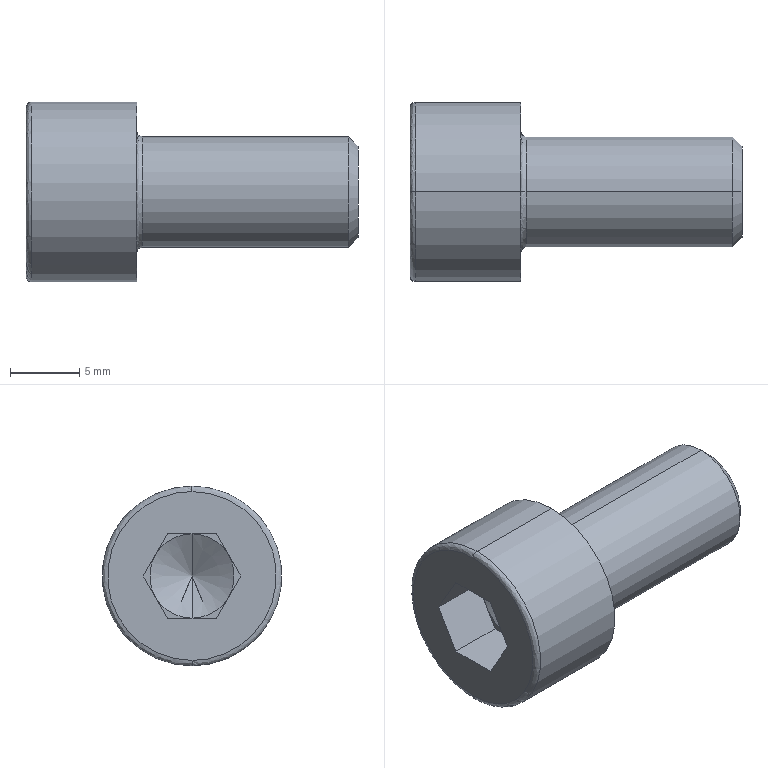Part | STEP file | PN_0040_default | 1 solid | 27 faces | box 24 x 13 x 13 mm | volume 1714 mm3 | plane 15 | spline 4 | cylinder 4 | cone 4 | commonest cylinder face diameters 8 x2 13 x2